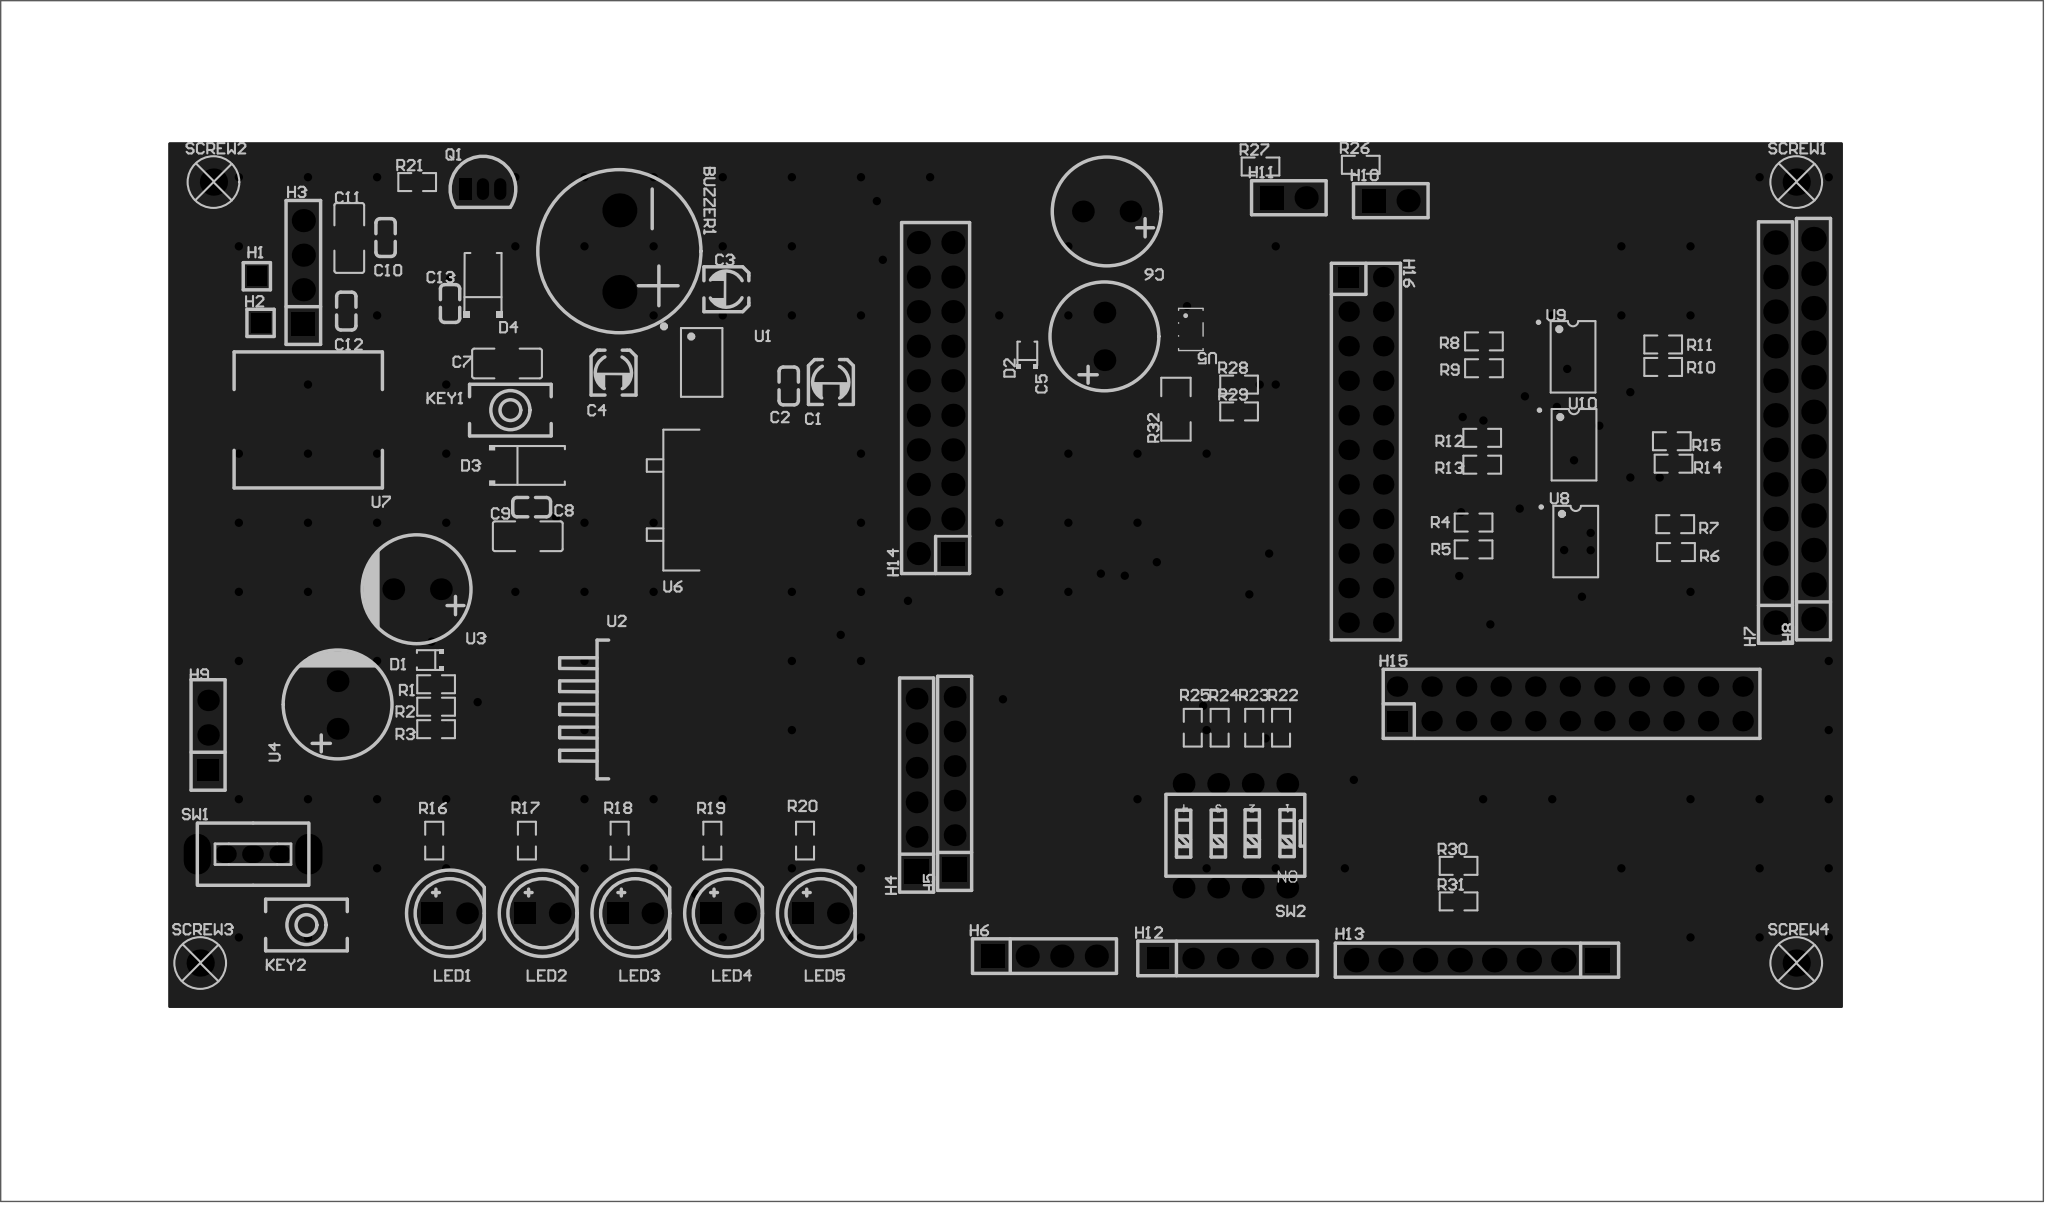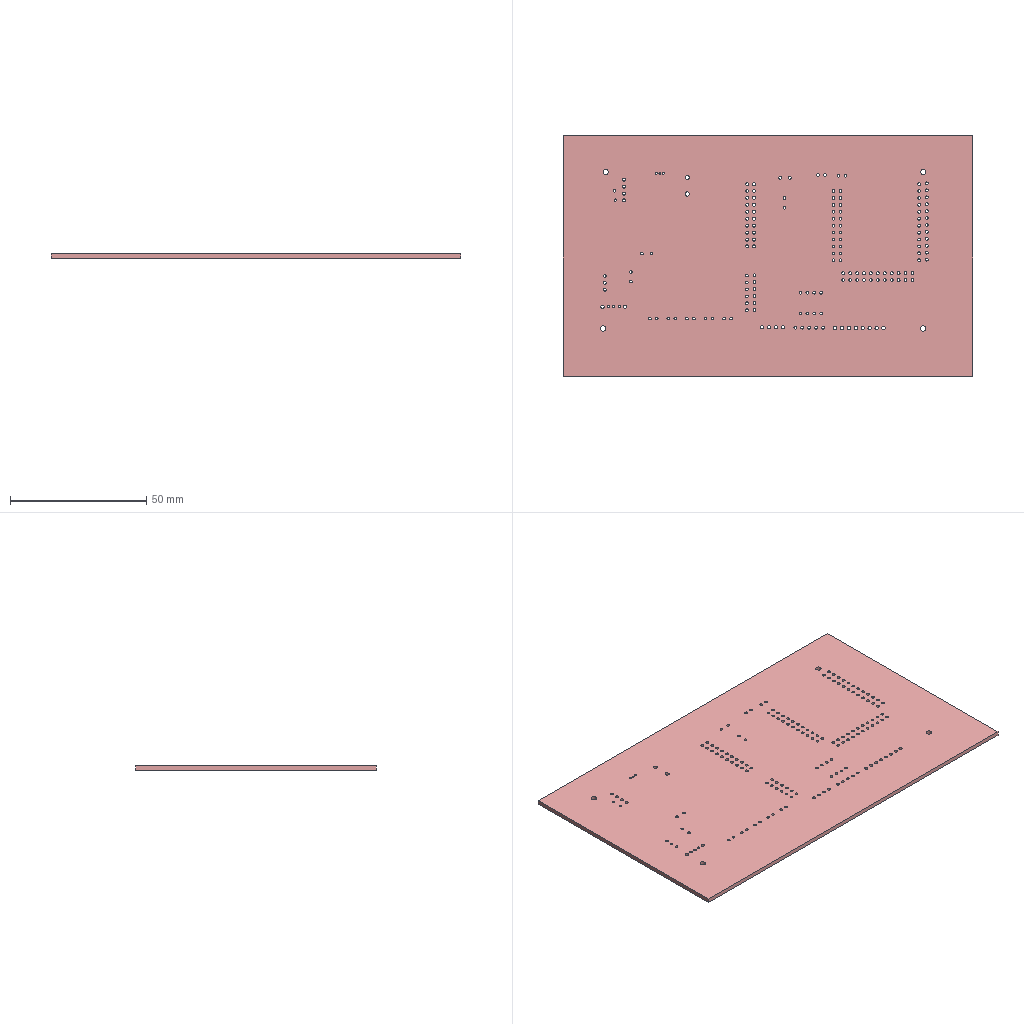Circuit board layout | Altium Designer | box 150.1 x 88.3 x 1.6 mm
Layer stack:
# Altium Designer layer stack of  (unit mm; dielectric type: 0 none, 1 core, 2 prepreg, 3 surface material)
index,name,kind,layer,copper_thickness_mm,dielectric_type,dielectric_thickness_mm,dielectric_material,dielectric_constant
0,Top Paste Mask Layer,other,,,,,,
1,Top Silkscreen Layer,other,,,,,,
2,Top Solder Mask Layer,dielectric,,,3,0,,0
3,Top Layer,copper,Top Layer,0.035,,,,
4,Dielectric1,dielectric,,,3,0.2104,7628 RC49% 8.6mil,0
5,Inner1,copper,Inner1,0.0152,,,,
6,Dielectric2,dielectric,,,3,1.065,1.1mm H/HOZ Copper,0
7,Inner2,copper,Inner2,0.0152,,,,
8,Dielectric3,dielectric,,,3,0.2104,7628 RC49% 8.6mil,0
9,Bottom Layer,copper,Bottom Layer,0.035,,,,
10,Bottom Solder Mask Layer,dielectric,,,3,0,,0
11,Bottom Silkscreen Layer,other,,,,,,
12,Bottom Paste Mask Layer,other,,,,,,
# drill layer pairs: low layer,high layer
drill_pair,Top Layer,Bottom Layer
Part placement:
Designator,Comment,Layer,Footprint,Center-X(mm),Center-Y(mm),Rotation
BUZZER1,buzzer,TopLayer,BUZ-TH_BD12.0-P6.00-D0.9-RD,115.316,139.7,270
C1,100uF,TopLayer,C_Ele_SMD_3x5.4mm,130.867,130.083,90
C2,100nF,TopLayer,C0603,127.762,129.794,270
C3,10uF,TopLayer,C_Ele_SMD_3x5.4mm,123.181,136.896,0
C4,47uF,TopLayer,C_Ele_SMD_3x5.4mm,114.893,130.774,90
C5,4.7uF,TopLayer,CAP-TH_BD8.0-P3.50-D0.5-FD_4.7UF400V8X14FS,150.963,133.438,90
C6,4.7uF,TopLayer,CAP-TH_BD8.0-P3.50-D0.5-FD_4.7UF400V8X14FS,151.13,142.621,180
C7,47UF,TopLayer,C1206,107.061,131.445,0
C8,100nF,TopLayer,C0603,108.87,120.885,0
C9,22UF,TopLayer,C1206,108.585,118.745,0
C10,100nF,TopLayer,C0603,98.135,140.702,90
C11,22UF,TopLayer,C1206,95.468,140.67,90
C12,4.7UF,TopLayer,C0603,95.247,135.297,270
C13,100nF,TopLayer,C0603,102.875,135.853,270
D1,1N5819WS,TopLayer,SOD-323_L1.8-W1.3-LS2.5-RD,101.34,109.645,180
D2,1N5819WS,TopLayer,SOD-323_L1.8-W1.3-LS2.5-RD,145.298,132.148,90
D3,SS34,TopLayer,SMA_L4.3-W2.6-LS5.2-RD,108.712,123.952,0
D4,SS34,TopLayer,SMA_L4.3-W2.6-LS5.0-RD,105.291,137.408,90
H1,,TopLayer,HDR-TH_1P-V-M_XKB_X4611WV-01I-C28D40,88.674,137.858,90
H2,,TopLayer,HDR-TH_1P-V-M_XKB_X4611WV-01I-C28D40,88.947,134.429,90
H3,,TopLayer,HDR-TH_4P-P2.54-V-F,92.091,138.137,90
H4,,TopLayer,HDR-TH_6P-P2.54-V-F,137.16,100.457,90
H5,,TopLayer,HDR-TH_6P-P2.54-V-F,139.954,100.584,90
H6,,TopLayer,HDR-TH_4P-P2.54-V-F,146.558,87.884,0
H7,,TopLayer,HDR-TH_12P-P2.54-V-F,200.279,126.365,90
H8,,TopLayer,HDR-TH_12P-P2.54-V-F,203.073,126.619,90
H9,,TopLayer,HDR-TH_3P-P2.54-V-F,85.09,104.14,90
H10,,TopLayer,HDR-TH_2P-P2.54-V-F,172.007,143.414,0
H11,,TopLayer,HDR-TH_2P-P2.54-V-F,164.514,143.627,0
H12,,TopLayer,HDR-TH_5P-P2.54-V-F,160.016,87.714,0
H13,,TopLayer,HDR-TH_8P-P2.54-V-F-1,178.339,87.587,180
H14,,TopLayer,HDR-TH_20P-P2.54-V-R2-C10-S2.54,138.557,128.905,90
H15,CS-1106-2*11B,TopLayer,HDR-TH_22P-P2.54-V-M-R2-C11-S2.54-1,185.166,106.426,0
H16,CS-1106-2*11B,TopLayer,HDR-TH_22P-P2.54-V-M-R2-C11-S2.54-1,170.18,125.095,270
KEY1,SW-SPST,TopLayer,KEY-SMD_L6.0-W3.6-LS8.0,107.315,128.016,0
KEY2,SW-SPST,TopLayer,KEY-SMD_L6.0-W3.6-LS8.0,92.329,90.17,0
LED1,,TopLayer,LED-TH_5mm,102.851,91.032,0
LED2,,TopLayer,LED-TH_5mm,109.665,91.032,0
LED3,,TopLayer,LED-TH_5mm,116.478,91.032,0
LED4,,TopLayer,LED-TH_5mm,123.291,91.032,0
LED5,,TopLayer,LED-TH_5mm,130.104,91.032,0
Q1,,TopLayer,S8050_TO_92,105.291,144.266,0
R1,3.9K,TopLayer,R0603,101.848,107.867,0
R2,1K,TopLayer,R0603,101.848,106.216,180
R3,1K,TopLayer,R0603,101.848,104.565,180
R4,1K,TopLayer,R0603,178.091,119.753,180
R5,1K,TopLayer,R0603,178.091,117.779,180
R6,1K,TopLayer,R0603,192.969,117.583,0
R7,1K,TopLayer,R0603,192.913,119.634,0
R8,1K,TopLayer,R0603,178.853,133.069,180
R9,1K,TopLayer,R0603,178.853,131.095,180
R10,1K,TopLayer,R0603,192.024,131.191,0
R11,1K,TopLayer,R0603,192.024,132.842,0
R12,1K,TopLayer,R0603,178.726,125.981,180
R13,1K,TopLayer,R0603,178.726,124.007,180
R14,1K,TopLayer,R0603,192.786,124.079,0
R15,1K,TopLayer,R0603,192.659,125.73,0
R16,1K,TopLayer,R0603,101.708,96.374,90
R17,1K,TopLayer,R0603,108.522,96.374,90
R18,1K,TopLayer,R0603,115.335,96.374,90
R19,3.3K,TopLayer,R0603,122.148,96.374,90
R20,3.3K,TopLayer,R0603,128.961,96.374,90
R21,1K,TopLayer,R0603,100.457,144.78,0
R22,1K,TopLayer,R0603,163.942,104.672,270
R23,1K,TopLayer,R0603,161.969,104.672,270
R24,1K,TopLayer,R0603,159.429,104.672,270
R25,1K,TopLayer,R0603,157.455,104.672,270
R26,1K,TopLayer,R0603,169.799,146.05,0
R27,1K,TopLayer,R0603,162.433,145.923,0
R28,1K,TopLayer,R0603,160.859,129.893,0
R29,1K,TopLayer,R0603,160.859,127.92,0
R30,1K,TopLayer,R0603,176.988,94.519,0
R31,1K,TopLayer,R0603,176.988,91.905,0
R32,100mΩ,TopLayer,R1206,156.219,128.085,90
SCREW1,,TopLayer,M2螺丝,201.803,144.78,0
SCREW2,,TopLayer,M2螺丝,85.487,144.78,0
SCREW3,,TopLayer,M2螺丝,84.511,87.376,0
SCREW4,,TopLayer,M2螺丝,201.803,87.376,0
SW1,,TopLayer,拨动开关,88.4,95.377,0
SW2,DIP switch EI-04,TopLayer,SW-TH_DIPSWITCHEI-04,160.591,96.73,180
U1,LM2663M,TopLayer,SOIC-8_L4.9-W3.9-P1.27-LS6.0-BL,121.365,131.522,270
U2,MIC29302,TopLayer,TO-263-5_L10.1-W8.7-P1.70-LS15.2-BR,114.078,106.014,180
U3,22UF400V,TopLayer,CAP-TH_BD8.0-P3.50-D0.6-FD,100.451,114.852,180
U4,22UF400V,TopLayer,CAP-TH_BD8.0-P3.50-D0.6-FD,94.609,106.343,90
U5,TPS73633DBVR,TopLayer,SOT-23-5_L3.0-W1.7-P0.95-LS2.8-BR,157.313,133.946,180
U6,LM2940HR-5.0,TopLayer,TO-263-2_L10.1-W9.1-P5.08-LS15.2-BR,120.452,121.404,180
U7,6.8UH,TopLayer,IND-SMD_L10.9-W10.0_ACL1009,92.453,127.296,180
U8,HCPL-0631-000E,TopLayer,SO-8_L5.1-W3.9-P1.27-LS6.0-BL,185.599,118.356,270
U9,HCPL-0631-000E,TopLayer,SO-8_L5.1-W3.9-P1.27-LS6.0-BL,185.401,131.934,270
U10,HCPL-0631-000E,TopLayer,SO-8_L5.1-W3.9-P1.27-LS6.0-BL,185.472,125.473,270
Pad and via stacks:
# Altium Designer via and pad stacks of  (unit mm). Each distinct definition once, with the count of objects using it.
# via: kind,start_layer,end_layer,hole_mm,diameter_mm,mode(0 simple;1 top-mid-bottom;2 full stack),diameter_per_layer,count,example_net
# pad: kind,layer,hole_mm,hole_type(0 round;1 square;2 slot),plating,top_size,top_shape(1 round;2 rect;3 octagon;9 rounded rect),mid_size,bottom_size,mode,footprint,size_per_layer,count,example
pad,Multi-Layer,1.5,0,plated,2.5x2.5,1,2.5x2.5,2.5x2.5,0,BUZ-TH_BD12.0-P6.00-D0.9-RD,,2,BUZZER1.1
pad,Multi-Layer,1,0,plated,1.6x1.6,1,1.6x1.6,1.6x1.6,0,CAP-TH_BD8.0-P3.50-D0.5-FD_4.7UF400V8X14FS,,4,C5.2
pad,Multi-Layer,0.9,0,plated,1.4x1.4,2,1.4x1.4,1.4x1.4,0,HDR-TH_1P-V-M_XKB_X4611WV-01I-C28D40,,2,H1.1
pad,Multi-Layer,1.1,0,plated,1.7x1.7,2,1.7x1.7,1.7x1.7,0,HDR-TH_4P-P2.54-V-F,,2,H3.1
pad,Multi-Layer,1.1,0,plated,1.7x1.7,1,1.7x1.7,1.7x1.7,0,HDR-TH_4P-P2.54-V-F,,6,H3.2
pad,Multi-Layer,1.02,0,plated,1.6x1.6,1,1.6x1.6,1.6x1.6,0,HDR-TH_6P-P2.54-V-F,,10,H4.6
pad,Multi-Layer,1.02,0,plated,1.8x1.8,2,1.8x1.8,1.8x1.8,0,HDR-TH_6P-P2.54-V-F,,2,H4.1
pad,Multi-Layer,1.05,0,plated,1.8x1.8,1,1.8x1.8,1.8x1.8,0,HDR-TH_12P-P2.54-V-F,,24,H7.1
pad,Multi-Layer,1.02,0,plated,1.575x1.575,1,1.575x1.575,1.575x1.575,0,HDR-TH_3P-P2.54-V-F,,2,H9.3
pad,Multi-Layer,1.02,0,plated,1.575x1.575,2,1.575x1.575,1.575x1.575,0,HDR-TH_3P-P2.54-V-F,,1,H9.1
pad,Multi-Layer,1,0,plated,1.7x1.7,2,1.7x1.7,1.7x1.7,0,HDR-TH_2P-P2.54-V-F,,2,H10.1
pad,Multi-Layer,1,0,plated,1.7x1.7,1,1.7x1.7,1.7x1.7,0,HDR-TH_2P-P2.54-V-F,,2,H10.2
pad,Multi-Layer,1.02,0,plated,1.575x1.575,1,1.575x1.575,1.575x1.575,0,HDR-TH_5P-P2.54-V-F,,4,H12.5
pad,Multi-Layer,1.02,0,plated,1.575x1.575,2,1.575x1.575,1.575x1.575,0,HDR-TH_5P-P2.54-V-F,,1,H12.1
pad,Multi-Layer,1.2,0,plated,1.8x1.8,2,1.8x1.8,1.8x1.8,0,HDR-TH_8P-P2.54-V-F-1,,1,H13.1
pad,Multi-Layer,1.2,0,plated,1.8x1.8,1,1.8x1.8,1.8x1.8,0,HDR-TH_8P-P2.54-V-F-1,,7,H13.2
pad,Multi-Layer,1.1,0,plated,1.7x1.7,1,1.7x1.7,1.7x1.7,0,HDR-TH_20P-P2.54-V-R2-C10-S2.54,,19,H14.20
pad,Multi-Layer,1.1,0,plated,1.7x1.7,2,1.7x1.7,1.7x1.7,0,HDR-TH_20P-P2.54-V-R2-C10-S2.54,,1,H14.1
pad,Multi-Layer,1,0,plated,1.5x1.5,2,1.5x1.5,1.5x1.5,0,HDR-TH_22P-P2.54-V-M-R2-C11-S2.54-1,,2,H15.1
pad,Multi-Layer,1,0,plated,1.5x1.5,1,1.5x1.5,1.5x1.5,0,HDR-TH_22P-P2.54-V-M-R2-C11-S2.54-1,,42,H15.2
pad,Multi-Layer,1,0,plated,1.6x1.6,2,1.6x1.6,1.6x1.6,0,LED-TH_5mm,,5,LED1.1
pad,Multi-Layer,1,0,plated,1.6x1.6,1,1.6x1.6,1.6x1.6,0,LED-TH_5mm,,5,LED1.2
pad,Multi-Layer,0.701,0,plated,0.8992x1.6,2,0.8992x1.6,0.8992x1.6,0,S8050_TO_92,,1,Q1.1
pad,Multi-Layer,0.701,0,plated,0.8992x1.6,1,0.8992x1.6,0.8992x1.6,0,S8050_TO_92,,2,Q1.2
pad,Multi-Layer,2,0,plated,2x2,1,2x2,2x2,0,M2\u00C2\u00DD\u00CB\u00BF,,4,SCREW1.1
pad,Multi-Layer,0.8992,0,plated,1.6x1.3,1,1.6x1.3,1.6x1.3,0,\u00B2\u00A6\u00B6\u00AF\u00BF\u00AA\u00B9\u00D8,,3,SW1.1
pad,Multi-Layer,1.3,0,plated,3x1.999,1,3x1.999,3x1.999,0,\u00B2\u00A6\u00B6\u00AF\u00BF\u00AA\u00B9\u00D8,,2,SW1.4
pad,Multi-Layer,1,0,plated,1.6x1.6,1,1.6x1.6,1.6x1.6,0,SW-TH_DIPSWITCHEI-04,,8,SW2.1
pad,Multi-Layer,1,0,plated,1.6x1.6,1,1.6x1.6,1.6x1.6,0,CAP-TH_BD8.0-P3.50-D0.6-FD,,4,U3.2
pad,Top Layer,0,0,plated,1.999x0.8001,2,1.999x0.8001,1.999x0.8001,0,C_Ele_SMD_3x5.4mm,,6,C1.1
pad,Top Layer,0,0,plated,0.8x0.9,2,0.8x0.9,0.8x0.9,0,C0603,,10,C2.2
pad,Top Layer,0,0,plated,1.485x1.728,2,1.485x1.728,1.485x1.728,0,C1206,,6,C7.2
pad,Top Layer,0,0,plated,1x0.75,2,1x0.75,1x0.75,0,SOD-323_L1.8-W1.3-LS2.5-RD,,4,D1.2
pad,Top Layer,0,0,plated,2x2,2,2x2,2x2,0,SMA_L4.3-W2.6-LS5.2-RD,,2,D3.2
pad,Top Layer,0,0,plated,2.046x1.62,2,2.046x1.62,2.046x1.62,0,SMA_L4.3-W2.6-LS5.0-RD,,2,D4.2
pad,Top Layer,0,0,plated,1.7x1.5,2,1.7x1.5,1.7x1.5,0,KEY-SMD_L6.0-W3.6-LS8.0,,4,KEY1.2
pad,Top Layer,0,0,plated,0.8065x0.864,2,0.8065x0.864,0.8065x0.864,0,R0603,,62,R1.2
pad,Top Layer,0,0,plated,1.208x1.701,2,1.208x1.701,1.208x1.701,0,R1206,,2,R32.2
pad,Top Layer,0,0,plated,0.588x2.045,1,0.588x2.045,0.588x2.045,0,SOIC-8_L4.9-W3.9-P1.27-LS6.0-BL,,8,U1.5
pad,Top Layer,0,0,plated,9x11,2,9x11,9x11,0,TO-263-5_L10.1-W8.7-P1.70-LS15.2-BR,,1,U2.6
pad,Top Layer,0,0,plated,3.358x1.02,2,3.358x1.02,3.358x1.02,0,TO-263-5_L10.1-W8.7-P1.70-LS15.2-BR,,5,U2.5
pad,Top Layer,0,0,plated,1.1x0.6,2,1.1x0.6,1.1x0.6,0,SOT-23-5_L3.0-W1.7-P0.95-LS2.8-BR,,5,U5.5
pad,Top Layer,0,0,plated,3.7x1.8,2,3.7x1.8,3.7x1.8,0,TO-263-2_L10.1-W9.1-P5.08-LS15.2-BR,,2,U6.1
pad,Top Layer,0,0,plated,8.4x10.608,2,8.4x10.608,8.4x10.608,0,TO-263-2_L10.1-W9.1-P5.08-LS15.2-BR,,1,U6.2
pad,Top Layer,0,0,plated,2.6x4,2,2.6x4,2.6x4,0,IND-SMD_L10.9-W10.0_ACL1009,,2,U7.1
pad,Top Layer,0,0,plated,0.5684x1.27,1,0.5684x1.27,0.5684x1.27,0,SO-8_L5.1-W3.9-P1.27-LS6.0-BL,,24,U8.1
via,Top Layer,Bottom Layer,0.3048,0.61,0,,149,C3
Copper pours:
name,layer,net,type(0 solid;1 hatched;2 none)
Top Layer-GND,Top Layer,GND,0
Bottom Layer-GND,Bottom Layer,GND,0
Inner1-GND,Inner1,GND,0
Inner2-GND,Inner2,GND,0
Design rules, without the lines most boards share:
# Altium Designer design rules of  (exported by Altium Designer, unit mm)
# columns: name | kind | enabled | priority | scope1 | scope2 | descriptor | typed fields (field=value)
copperThickness1oz_2 | 2 | enabled | 2 | All | All | Width Constraint (Min=5mil) (Max=100mil) (Preferred=30mil) (All) |